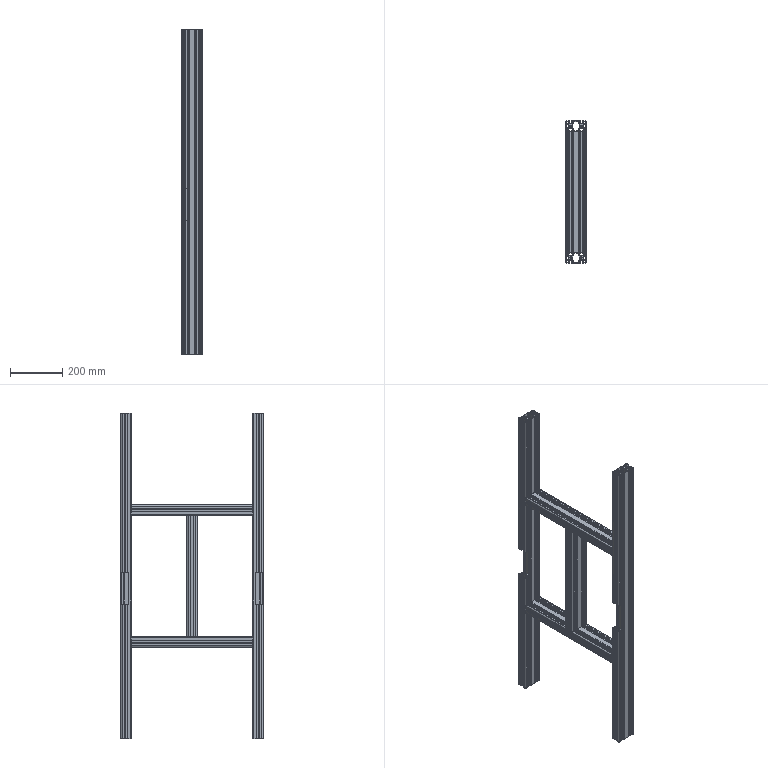Part | SolidWorks | features BaseBody 5 | 5 solids | 986 faces | box 80 x 545 x 1250 mm | volume 4052251 mm3 | plane 822 | cylinder 164 | commonest cylinder face diameters 2 x92 10 x48 6.5 x24